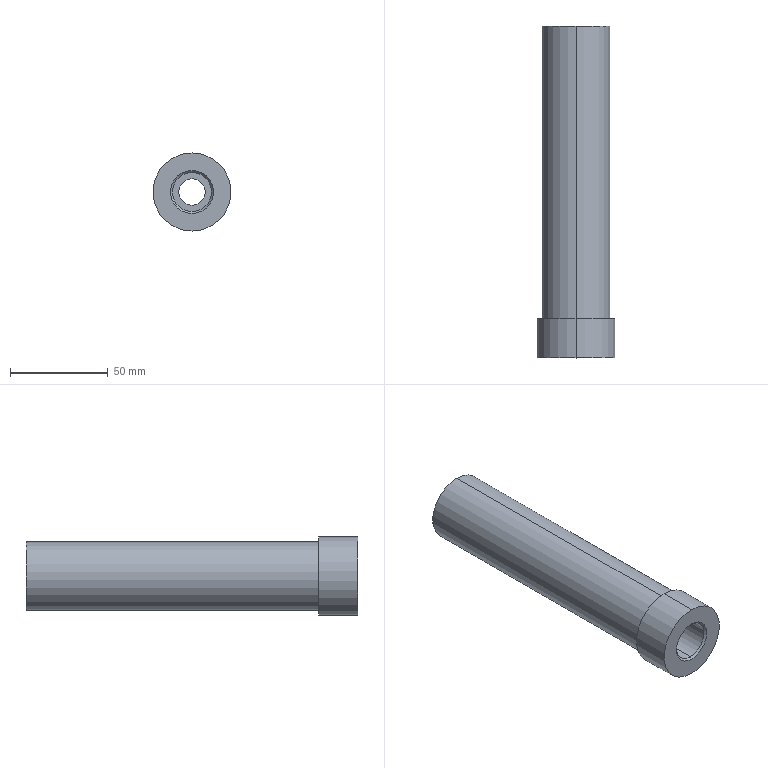Part | STEP file | 1 solid | 14 faces | box 40 x 170 x 40 mm | volume 118148 mm3 | cylinder 8 | plane 4 | cone 2 | commonest cylinder face diameters 13.5 x2 20 x2 35 x2 40 x2
STEP:
#1=CARTESIAN_POINT('',(0.,0.,0.));
#2=DIRECTION('',(0.,0.,1.));
#3=DIRECTION('',(1.,0.,0.));
#4=AXIS2_PLACEMENT_3D('',#1,#2,#3);
#5=CARTESIAN_POINT('',(-72.862,-219.,163.53));
#6=VERTEX_POINT('',#5);
#7=CARTESIAN_POINT('',(-72.862,-220.,162.53));
#8=VERTEX_POINT('',#7);
#9=CARTESIAN_POINT('',(-72.862,-220.,162.53));
#10=DIRECTION('',(0.,-0.7071,-0.7071));
#11=VECTOR('',#10,1.);
#12=LINE('',#9,#11);
#13=CARTESIAN_POINT('',(-72.862,-220.,173.53));
#14=DIRECTION('',(0.,-1.,0.));
#15=DIRECTION('',(0.,0.,-1.));
#16=AXIS2_PLACEMENT_3D('',#13,#14,#15);
#17=CONICAL_SURFACE('',#16,11.,0.7854);
#18=CARTESIAN_POINT('',(6.283,0.));
#19=DIRECTION('',(0.,1.));
#20=VECTOR('',#19,1.);
#21=LINE('',#18,#20);
#22=(GEOMETRIC_REPRESENTATION_CONTEXT(2)PARAMETRIC_REPRESENTATION_CONTEXT()REPRESENTATION_CONTEXT('',''));
#23=DEFINITIONAL_REPRESENTATION('',(#21),#22);
#24=PCURVE('',#17,#23);
#25=CARTESIAN_POINT('',(-72.862,-220.,173.53));
#26=DIRECTION('',(0.,-1.,0.));
#27=DIRECTION('',(0.,0.,-1.));
#28=AXIS2_PLACEMENT_3D('',#25,#26,#27);
#29=CONICAL_SURFACE('',#28,11.,0.7854);
#30=CARTESIAN_POINT('',(0.,0.));
#31=DIRECTION('',(0.,1.));
#32=VECTOR('',#31,1.);
#33=LINE('',#30,#32);
#34=(GEOMETRIC_REPRESENTATION_CONTEXT(2)PARAMETRIC_REPRESENTATION_CONTEXT()REPRESENTATION_CONTEXT('',''));
#35=DEFINITIONAL_REPRESENTATION('',(#33),#34);
#36=PCURVE('',#29,#35);
#37=SURFACE_CURVE('',#12,(#24,#36),.PCURVE_S1.);
#38=EDGE_CURVE('',#6,#8,#37,.T.);
#39=ORIENTED_EDGE('',*,*,#38,.T.);
#40=CARTESIAN_POINT('',(-72.862,-220.,184.53));
#41=VERTEX_POINT('',#40);
#42=CARTESIAN_POINT('',(-72.862,-220.,173.53));
#43=DIRECTION('',(0.,1.,0.));
#44=DIRECTION('',(0.,0.,-1.));
#45=AXIS2_PLACEMENT_3D('',#42,#43,#44);
#46=CIRCLE('',#45,11.);
#47=CARTESIAN_POINT('',(6.283,0.));
#48=DIRECTION('',(-1.,0.));
#49=VECTOR('',#48,1.);
#50=LINE('',#47,#49);
#51=(GEOMETRIC_REPRESENTATION_CONTEXT(2)PARAMETRIC_REPRESENTATION_CONTEXT()REPRESENTATION_CONTEXT('',''));
#52=DEFINITIONAL_REPRESENTATION('',(#50),#51);
#53=PCURVE('',#17,#52);
#54=CARTESIAN_POINT('',(-72.862,-220.,173.53));
#55=DIRECTION('',(0.,-1.,0.));
#56=DIRECTION('',(0.,0.,-1.));
#57=AXIS2_PLACEMENT_3D('',#54,#55,#56);
#58=PLANE('',#57);
#59=CARTESIAN_POINT('',(11.,0.));
#60=CARTESIAN_POINT('',(11.,-19.053));
#61=CARTESIAN_POINT('',(-5.5,-9.526));
#62=CARTESIAN_POINT('',(-22.,0.));
#63=CARTESIAN_POINT('',(-5.5,9.526));
#64=CARTESIAN_POINT('',(11.,19.053));
#65=CARTESIAN_POINT('',(11.,0.));
#66=(BOUNDED_CURVE()B_SPLINE_CURVE(2,(#59,#60,#61,#62,#63,#64,#65),.UNSPECIFIED.,.T.,.F.)B_SPLINE_CURVE_WITH_KNOTS((1,2,2,2,2,1),(-2.094,0.,2.094,4.189,6.283,8.378),.UNSPECIFIED.)CURVE()GEOMETRIC_REPRESENTATION_ITEM()RATIONAL_B_SPLINE_CURVE((1.,0.5,1.,0.5,1.,0.5,1.))REPRESENTATION_ITEM(''));
#67=(GEOMETRIC_REPRESENTATION_CONTEXT(2)PARAMETRIC_REPRESENTATION_CONTEXT()REPRESENTATION_CONTEXT('',''));
#68=DEFINITIONAL_REPRESENTATION('',(#66),#67);
#69=PCURVE('',#58,#68);
#70=SURFACE_CURVE('',#46,(#53,#69),.PCURVE_S1.);
#71=EDGE_CURVE('',#8,#41,#70,.T.);
#72=ORIENTED_EDGE('',*,*,#71,.T.);
#73=CARTESIAN_POINT('',(-72.862,-219.,183.53));
#74=VERTEX_POINT('',#73);
#75=CARTESIAN_POINT('',(-72.862,-220.,184.53));
#76=DIRECTION('',(0.,-0.7071,0.7071));
#77=VECTOR('',#76,1.);
#78=LINE('',#75,#77);
#79=CARTESIAN_POINT('',(3.142,0.));
#80=DIRECTION('',(0.,1.));
#81=VECTOR('',#80,1.);
#82=LINE('',#79,#81);
#83=(GEOMETRIC_REPRESENTATION_CONTEXT(2)PARAMETRIC_REPRESENTATION_CONTEXT()REPRESENTATION_CONTEXT('',''));
#84=DEFINITIONAL_REPRESENTATION('',(#82),#83);
#85=PCURVE('',#17,#84);
#86=CARTESIAN_POINT('',(3.142,0.));
#87=DIRECTION('',(0.,1.));
#88=VECTOR('',#87,1.);
#89=LINE('',#86,#88);
#90=(GEOMETRIC_REPRESENTATION_CONTEXT(2)PARAMETRIC_REPRESENTATION_CONTEXT()REPRESENTATION_CONTEXT('',''));
#91=DEFINITIONAL_REPRESENTATION('',(#89),#90);
#92=PCURVE('',#29,#91);
#93=SURFACE_CURVE('',#78,(#85,#92),.PCURVE_S1.);
#94=EDGE_CURVE('',#74,#41,#93,.T.);
#95=ORIENTED_EDGE('',*,*,#94,.F.);
#96=CARTESIAN_POINT('',(-72.862,-219.,173.53));
#97=DIRECTION('',(0.,-1.,0.));
#98=DIRECTION('',(0.,0.,-1.));
#99=AXIS2_PLACEMENT_3D('',#96,#97,#98);
#100=CIRCLE('',#99,10.);
#101=CARTESIAN_POINT('',(0.,-1.));
#102=DIRECTION('',(1.,0.));
#103=VECTOR('',#102,1.);
#104=LINE('',#101,#103);
#105=(GEOMETRIC_REPRESENTATION_CONTEXT(2)PARAMETRIC_REPRESENTATION_CONTEXT()REPRESENTATION_CONTEXT('',''));
#106=DEFINITIONAL_REPRESENTATION('',(#104),#105);
#107=PCURVE('',#17,#106);
#108=CARTESIAN_POINT('',(-72.862,-220.,173.53));
#109=DIRECTION('',(0.,1.,0.));
#110=DIRECTION('',(0.,0.,1.));
#111=AXIS2_PLACEMENT_3D('',#108,#109,#110);
#112=CYLINDRICAL_SURFACE('',#111,10.);
#113=CARTESIAN_POINT('',(9.425,1.));
#114=DIRECTION('',(-1.,0.));
#115=VECTOR('',#114,1.);
#116=LINE('',#113,#115);
#117=(GEOMETRIC_REPRESENTATION_CONTEXT(2)PARAMETRIC_REPRESENTATION_CONTEXT()REPRESENTATION_CONTEXT('',''));
#118=DEFINITIONAL_REPRESENTATION('',(#116),#117);
#119=PCURVE('',#112,#118);
#120=SURFACE_CURVE('',#100,(#107,#119),.PCURVE_S1.);
#121=EDGE_CURVE('',#74,#6,#120,.T.);
#122=ORIENTED_EDGE('',*,*,#121,.T.);
#123=EDGE_LOOP('',(#39,#72,#95,#122));
#124=FACE_BOUND('',#123,.F.);
#125=ADVANCED_FACE('',(#124),#17,.F.);
#126=CARTESIAN_POINT('',(-72.862,-62.5,183.53));
#127=VERTEX_POINT('',#126);
#128=CARTESIAN_POINT('',(-72.862,-220.,183.53));
#129=DIRECTION('',(0.,1.,0.));
#130=VECTOR('',#129,1.);
#131=LINE('',#128,#130);
#132=CARTESIAN_POINT('',(6.283,0.));
#133=DIRECTION('',(0.,1.));
#134=VECTOR('',#133,1.);
#135=LINE('',#132,#134);
#136=(GEOMETRIC_REPRESENTATION_CONTEXT(2)PARAMETRIC_REPRESENTATION_CONTEXT()REPRESENTATION_CONTEXT('',''));
#137=DEFINITIONAL_REPRESENTATION('',(#135),#136);
#138=PCURVE('',#112,#137);
#139=CARTESIAN_POINT('',(-72.862,-220.,173.53));
#140=DIRECTION('',(0.,1.,0.));
#141=DIRECTION('',(0.,0.,1.));
#142=AXIS2_PLACEMENT_3D('',#139,#140,#141);
#143=CYLINDRICAL_SURFACE('',#142,10.);
#144=CARTESIAN_POINT('',(0.,0.));
#145=DIRECTION('',(0.,1.));
#146=VECTOR('',#145,1.);
#147=LINE('',#144,#146);
#148=(GEOMETRIC_REPRESENTATION_CONTEXT(2)PARAMETRIC_REPRESENTATION_CONTEXT()REPRESENTATION_CONTEXT('',''));
#149=DEFINITIONAL_REPRESENTATION('',(#147),#148);
#150=PCURVE('',#143,#149);
#151=SURFACE_CURVE('',#131,(#138,#150),.PCURVE_S1.);
#152=EDGE_CURVE('',#74,#127,#151,.T.);
#153=ORIENTED_EDGE('',*,*,#152,.T.);
#154=CARTESIAN_POINT('',(-72.862,-62.5,163.53));
#155=VERTEX_POINT('',#154);
#156=CARTESIAN_POINT('',(-72.862,-62.5,173.53));
#157=DIRECTION('',(0.,-1.,0.));
#158=DIRECTION('',(0.,0.,1.));
#159=AXIS2_PLACEMENT_3D('',#156,#157,#158);
#160=CIRCLE('',#159,10.);
#161=CARTESIAN_POINT('',(6.283,157.5));
#162=DIRECTION('',(-1.,0.));
#163=VECTOR('',#162,1.);
#164=LINE('',#161,#163);
#165=(GEOMETRIC_REPRESENTATION_CONTEXT(2)PARAMETRIC_REPRESENTATION_CONTEXT()REPRESENTATION_CONTEXT('',''));
#166=DEFINITIONAL_REPRESENTATION('',(#164),#165);
#167=PCURVE('',#112,#166);
#168=CARTESIAN_POINT('',(-72.862,-62.5,173.53));
#169=DIRECTION('',(0.,1.,0.));
#170=DIRECTION('',(0.,0.,1.));
#171=AXIS2_PLACEMENT_3D('',#168,#169,#170);
#172=PLANE('',#171);
#173=CARTESIAN_POINT('',(10.,0.));
#174=CARTESIAN_POINT('',(10.,-17.321));
#175=CARTESIAN_POINT('',(-5.,-8.66));
#176=CARTESIAN_POINT('',(-20.,0.));
#177=CARTESIAN_POINT('',(-5.,8.66));
#178=CARTESIAN_POINT('',(10.,17.321));
#179=CARTESIAN_POINT('',(10.,0.));
#180=(BOUNDED_CURVE()B_SPLINE_CURVE(2,(#173,#174,#175,#176,#177,#178,#179),.UNSPECIFIED.,.T.,.F.)B_SPLINE_CURVE_WITH_KNOTS((1,2,2,2,2,1),(-2.094,0.,2.094,4.189,6.283,8.378),.UNSPECIFIED.)CURVE()GEOMETRIC_REPRESENTATION_ITEM()RATIONAL_B_SPLINE_CURVE((1.,0.5,1.,0.5,1.,0.5,1.))REPRESENTATION_ITEM(''));
#181=(GEOMETRIC_REPRESENTATION_CONTEXT(2)PARAMETRIC_REPRESENTATION_CONTEXT()REPRESENTATION_CONTEXT('',''));
#182=DEFINITIONAL_REPRESENTATION('',(#180),#181);
#183=PCURVE('',#172,#182);
#184=SURFACE_CURVE('',#160,(#167,#183),.PCURVE_S1.);
#185=EDGE_CURVE('',#127,#155,#184,.T.);
#186=ORIENTED_EDGE('',*,*,#185,.T.);
#187=CARTESIAN_POINT('',(-72.862,-220.,163.53));
#188=DIRECTION('',(0.,1.,0.));
#189=VECTOR('',#188,1.);
#190=LINE('',#187,#189);
#191=CARTESIAN_POINT('',(3.142,0.));
#192=DIRECTION('',(0.,1.));
#193=VECTOR('',#192,1.);
#194=LINE('',#191,#193);
#195=(GEOMETRIC_REPRESENTATION_CONTEXT(2)PARAMETRIC_REPRESENTATION_CONTEXT()REPRESENTATION_CONTEXT('',''));
#196=DEFINITIONAL_REPRESENTATION('',(#194),#195);
#197=PCURVE('',#112,#196);
#198=CARTESIAN_POINT('',(3.142,0.));
#199=DIRECTION('',(0.,1.));
#200=VECTOR('',#199,1.);
#201=LINE('',#198,#200);
#202=(GEOMETRIC_REPRESENTATION_CONTEXT(2)PARAMETRIC_REPRESENTATION_CONTEXT()REPRESENTATION_CONTEXT('',''));
#203=DEFINITIONAL_REPRESENTATION('',(#201),#202);
#204=PCURVE('',#143,#203);
#205=SURFACE_CURVE('',#190,(#197,#204),.PCURVE_S1.);
#206=EDGE_CURVE('',#6,#155,#205,.T.);
#207=ORIENTED_EDGE('',*,*,#206,.F.);
#208=ORIENTED_EDGE('',*,*,#121,.F.);
#209=EDGE_LOOP('',(#153,#186,#207,#208));
#210=FACE_BOUND('',#209,.F.);
#211=ADVANCED_FACE('',(#210),#112,.F.);
#212=CARTESIAN_POINT('',(-72.862,-62.5,180.28));
#213=VERTEX_POINT('',#212);
#214=CARTESIAN_POINT('',(-72.862,-50.,180.28));
#215=VERTEX_POINT('',#214);
#216=CARTESIAN_POINT('',(-72.862,-220.,180.28));
#217=DIRECTION('',(0.,1.,0.));
#218=VECTOR('',#217,1.);
#219=LINE('',#216,#218);
#220=CARTESIAN_POINT('',(-72.862,-220.,173.53));
#221=DIRECTION('',(0.,1.,0.));
#222=DIRECTION('',(0.,0.,1.));
#223=AXIS2_PLACEMENT_3D('',#220,#221,#222);
#224=CYLINDRICAL_SURFACE('',#223,6.75);
#225=CARTESIAN_POINT('',(6.283,0.));
#226=DIRECTION('',(0.,1.));
#227=VECTOR('',#226,1.);
#228=LINE('',#225,#227);
#229=(GEOMETRIC_REPRESENTATION_CONTEXT(2)PARAMETRIC_REPRESENTATION_CONTEXT()REPRESENTATION_CONTEXT('',''));
#230=DEFINITIONAL_REPRESENTATION('',(#228),#229);
#231=PCURVE('',#224,#230);
#232=CARTESIAN_POINT('',(-72.862,-220.,173.53));
#233=DIRECTION('',(0.,1.,0.));
#234=DIRECTION('',(0.,0.,1.));
#235=AXIS2_PLACEMENT_3D('',#232,#233,#234);
#236=CYLINDRICAL_SURFACE('',#235,6.75);
#237=CARTESIAN_POINT('',(0.,0.));
#238=DIRECTION('',(0.,1.));
#239=VECTOR('',#238,1.);
#240=LINE('',#237,#239);
#241=(GEOMETRIC_REPRESENTATION_CONTEXT(2)PARAMETRIC_REPRESENTATION_CONTEXT()REPRESENTATION_CONTEXT('',''));
#242=DEFINITIONAL_REPRESENTATION('',(#240),#241);
#243=PCURVE('',#236,#242);
#244=SURFACE_CURVE('',#219,(#231,#243),.PCURVE_S1.);
#245=EDGE_CURVE('',#213,#215,#244,.T.);
#246=ORIENTED_EDGE('',*,*,#245,.T.);
#247=CARTESIAN_POINT('',(-72.862,-50.,166.78));
#248=VERTEX_POINT('',#247);
#249=CARTESIAN_POINT('',(-72.862,-50.,173.53));
#250=DIRECTION('',(0.,1.,0.));
#251=DIRECTION('',(0.,0.,1.));
#252=AXIS2_PLACEMENT_3D('',#249,#250,#251);
#253=CIRCLE('',#252,6.75);
#254=CARTESIAN_POINT('',(0.,170.));
#255=DIRECTION('',(1.,0.));
#256=VECTOR('',#255,1.);
#257=LINE('',#254,#256);
#258=(GEOMETRIC_REPRESENTATION_CONTEXT(2)PARAMETRIC_REPRESENTATION_CONTEXT()REPRESENTATION_CONTEXT('',''));
#259=DEFINITIONAL_REPRESENTATION('',(#257),#258);
#260=PCURVE('',#224,#259);
#261=CARTESIAN_POINT('',(-72.862,-50.,173.53));
#262=DIRECTION('',(0.,1.,0.));
#263=DIRECTION('',(0.,0.,1.));
#264=AXIS2_PLACEMENT_3D('',#261,#262,#263);
#265=PLANE('',#264);
#266=CARTESIAN_POINT('',(0.,0.));
#267=DIRECTION('',(1.,0.));
#268=AXIS2_PLACEMENT_2D('',#266,#267);
#269=CIRCLE('',#268,6.75);
#270=(GEOMETRIC_REPRESENTATION_CONTEXT(2)PARAMETRIC_REPRESENTATION_CONTEXT()REPRESENTATION_CONTEXT('',''));
#271=DEFINITIONAL_REPRESENTATION('',(#269),#270);
#272=PCURVE('',#265,#271);
#273=SURFACE_CURVE('',#253,(#260,#272),.PCURVE_S1.);
#274=EDGE_CURVE('',#248,#215,#273,.T.);
#275=ORIENTED_EDGE('',*,*,#274,.F.);
#276=CARTESIAN_POINT('',(-72.862,-62.5,166.78));
#277=VERTEX_POINT('',#276);
#278=CARTESIAN_POINT('',(-72.862,-220.,166.78));
#279=DIRECTION('',(0.,1.,0.));
#280=VECTOR('',#279,1.);
#281=LINE('',#278,#280);
#282=CARTESIAN_POINT('',(3.142,0.));
#283=DIRECTION('',(0.,1.));
#284=VECTOR('',#283,1.);
#285=LINE('',#282,#284);
#286=(GEOMETRIC_REPRESENTATION_CONTEXT(2)PARAMETRIC_REPRESENTATION_CONTEXT()REPRESENTATION_CONTEXT('',''));
#287=DEFINITIONAL_REPRESENTATION('',(#285),#286);
#288=PCURVE('',#224,#287);
#289=CARTESIAN_POINT('',(3.142,0.));
#290=DIRECTION('',(0.,1.));
#291=VECTOR('',#290,1.);
#292=LINE('',#289,#291);
#293=(GEOMETRIC_REPRESENTATION_CONTEXT(2)PARAMETRIC_REPRESENTATION_CONTEXT()REPRESENTATION_CONTEXT('',''));
#294=DEFINITIONAL_REPRESENTATION('',(#292),#293);
#295=PCURVE('',#236,#294);
#296=SURFACE_CURVE('',#281,(#288,#295),.PCURVE_S1.);
#297=EDGE_CURVE('',#277,#248,#296,.T.);
#298=ORIENTED_EDGE('',*,*,#297,.F.);
#299=CARTESIAN_POINT('',(-72.862,-62.5,173.53));
#300=DIRECTION('',(0.,-1.,0.));
#301=DIRECTION('',(0.,0.,1.));
#302=AXIS2_PLACEMENT_3D('',#299,#300,#301);
#303=CIRCLE('',#302,6.75);
#304=CARTESIAN_POINT('',(6.283,157.5));
#305=DIRECTION('',(-1.,0.));
#306=VECTOR('',#305,1.);
#307=LINE('',#304,#306);
#308=(GEOMETRIC_REPRESENTATION_CONTEXT(2)PARAMETRIC_REPRESENTATION_CONTEXT()REPRESENTATION_CONTEXT('',''));
#309=DEFINITIONAL_REPRESENTATION('',(#307),#308);
#310=PCURVE('',#224,#309);
#311=CARTESIAN_POINT('',(6.75,0.));
#312=CARTESIAN_POINT('',(6.75,-11.691));
#313=CARTESIAN_POINT('',(-3.375,-5.846));
#314=CARTESIAN_POINT('',(-13.5,0.));
#315=CARTESIAN_POINT('',(-3.375,5.846));
#316=CARTESIAN_POINT('',(6.75,11.691));
#317=CARTESIAN_POINT('',(6.75,0.));
#318=(BOUNDED_CURVE()B_SPLINE_CURVE(2,(#311,#312,#313,#314,#315,#316,#317),.UNSPECIFIED.,.T.,.F.)B_SPLINE_CURVE_WITH_KNOTS((1,2,2,2,2,1),(-2.094,0.,2.094,4.189,6.283,8.378),.UNSPECIFIED.)CURVE()GEOMETRIC_REPRESENTATION_ITEM()RATIONAL_B_SPLINE_CURVE((1.,0.5,1.,0.5,1.,0.5,1.))REPRESENTATION_ITEM(''));
#319=(GEOMETRIC_REPRESENTATION_CONTEXT(2)PARAMETRIC_REPRESENTATION_CONTEXT()REPRESENTATION_CONTEXT('',''));
#320=DEFINITIONAL_REPRESENTATION('',(#318),#319);
#321=PCURVE('',#172,#320);
#322=SURFACE_CURVE('',#303,(#310,#321),.PCURVE_S1.);
#323=EDGE_CURVE('',#213,#277,#322,.T.);
#324=ORIENTED_EDGE('',*,*,#323,.F.);
#325=EDGE_LOOP('',(#246,#275,#298,#324));
#326=FACE_BOUND('',#325,.F.);
#327=ADVANCED_FACE('',(#326),#224,.F.);
#328=CARTESIAN_POINT('',(-72.862,-200.,193.53));
#329=VERTEX_POINT('',#328);
#330=CARTESIAN_POINT('',(-72.862,-200.,153.53));
#331=VERTEX_POINT('',#330);
#332=CARTESIAN_POINT('',(-72.862,-200.,173.53));
#333=DIRECTION('',(0.,1.,0.));
#334=DIRECTION('',(0.,0.,-1.));
#335=AXIS2_PLACEMENT_3D('',#332,#333,#334);
#336=CIRCLE('',#335,20.);
#337=CARTESIAN_POINT('',(-72.862,-50.,173.53));
#338=DIRECTION('',(0.,-1.,0.));
#339=DIRECTION('',(0.,0.,-1.));
#340=AXIS2_PLACEMENT_3D('',#337,#338,#339);
#341=CYLINDRICAL_SURFACE('',#340,20.);
#342=CARTESIAN_POINT('',(6.283,150.));
#343=DIRECTION('',(-1.,0.));
#344=VECTOR('',#343,1.);
#345=LINE('',#342,#344);
#346=(GEOMETRIC_REPRESENTATION_CONTEXT(2)PARAMETRIC_REPRESENTATION_CONTEXT()REPRESENTATION_CONTEXT('',''));
#347=DEFINITIONAL_REPRESENTATION('',(#345),#346);
#348=PCURVE('',#341,#347);
#349=CARTESIAN_POINT('',(-72.862,-200.,48.53));
#350=DIRECTION('',(0.,-1.,0.));
#351=DIRECTION('',(0.,0.,-1.));
#352=AXIS2_PLACEMENT_3D('',#349,#350,#351);
#353=PLANE('',#352);
#354=CARTESIAN_POINT('',(-105.,0.));
#355=CARTESIAN_POINT('',(-105.,-34.641));
#356=CARTESIAN_POINT('',(-135.,-17.321));
#357=CARTESIAN_POINT('',(-165.,0.));
#358=CARTESIAN_POINT('',(-135.,17.321));
#359=CARTESIAN_POINT('',(-105.,34.641));
#360=CARTESIAN_POINT('',(-105.,0.));
#361=(BOUNDED_CURVE()B_SPLINE_CURVE(2,(#354,#355,#356,#357,#358,#359,#360),.UNSPECIFIED.,.T.,.F.)B_SPLINE_CURVE_WITH_KNOTS((1,2,2,2,2,1),(-2.094,0.,2.094,4.189,6.283,8.378),.UNSPECIFIED.)CURVE()GEOMETRIC_REPRESENTATION_ITEM()RATIONAL_B_SPLINE_CURVE((1.,0.5,1.,0.5,1.,0.5,1.))REPRESENTATION_ITEM(''));
#362=(GEOMETRIC_REPRESENTATION_CONTEXT(2)PARAMETRIC_REPRESENTATION_CONTEXT()REPRESENTATION_CONTEXT('',''));
#363=DEFINITIONAL_REPRESENTATION('',(#361),#362);
#364=PCURVE('',#353,#363);
#365=SURFACE_CURVE('',#336,(#348,#364),.PCURVE_S1.);
#366=EDGE_CURVE('',#329,#331,#365,.T.);
#367=ORIENTED_EDGE('',*,*,#366,.F.);
#368=CARTESIAN_POINT('',(-72.862,-220.,193.53));
#369=VERTEX_POINT('',#368);
#370=CARTESIAN_POINT('',(-72.862,-50.,193.53));
#371=DIRECTION('',(0.,-1.,0.));
#372=VECTOR('',#371,1.);
#373=LINE('',#370,#372);
#374=CARTESIAN_POINT('',(3.142,0.));
#375=DIRECTION('',(0.,1.));
#376=VECTOR('',#375,1.);
#377=LINE('',#374,#376);
#378=(GEOMETRIC_REPRESENTATION_CONTEXT(2)PARAMETRIC_REPRESENTATION_CONTEXT()REPRESENTATION_CONTEXT('',''));
#379=DEFINITIONAL_REPRESENTATION('',(#377),#378);
#380=PCURVE('',#341,#379);
#381=CARTESIAN_POINT('',(-72.862,-50.,173.53));
#382=DIRECTION('',(0.,-1.,0.));
#383=DIRECTION('',(0.,0.,-1.));
#384=AXIS2_PLACEMENT_3D('',#381,#382,#383);
#385=CYLINDRICAL_SURFACE('',#384,20.);
#386=CARTESIAN_POINT('',(3.142,0.));
#387=DIRECTION('',(0.,1.));
#388=VECTOR('',#387,1.);
#389=LINE('',#386,#388);
#390=(GEOMETRIC_REPRESENTATION_CONTEXT(2)PARAMETRIC_REPRESENTATION_CONTEXT()REPRESENTATION_CONTEXT('',''));
#391=DEFINITIONAL_REPRESENTATION('',(#389),#390);
#392=PCURVE('',#385,#391);
#393=SURFACE_CURVE('',#373,(#380,#392),.PCURVE_S1.);
#394=EDGE_CURVE('',#329,#369,#393,.T.);
#395=ORIENTED_EDGE('',*,*,#394,.T.);
#396=CARTESIAN_POINT('',(-72.862,-220.,153.53));
#397=VERTEX_POINT('',#396);
#398=CARTESIAN_POINT('',(-72.862,-220.,173.53));
#399=DIRECTION('',(0.,-1.,0.));
#400=DIRECTION('',(0.,0.,-1.));
#401=AXIS2_PLACEMENT_3D('',#398,#399,#400);
#402=CIRCLE('',#401,20.);
#403=CARTESIAN_POINT('',(0.,170.));
#404=DIRECTION('',(1.,0.));
#405=VECTOR('',#404,1.);
#406=LINE('',#403,#405);
#407=(GEOMETRIC_REPRESENTATION_CONTEXT(2)PARAMETRIC_REPRESENTATION_CONTEXT()REPRESENTATION_CONTEXT('',''));
#408=DEFINITIONAL_REPRESENTATION('',(#406),#407);
#409=PCURVE('',#341,#408);
#410=CARTESIAN_POINT('',(0.,0.));
#411=DIRECTION('',(1.,0.));
#412=AXIS2_PLACEMENT_2D('',#410,#411);
#413=CIRCLE('',#412,20.);
#414=(GEOMETRIC_REPRESENTATION_CONTEXT(2)PARAMETRIC_REPRESENTATION_CONTEXT()REPRESENTATION_CONTEXT('',''));
#415=DEFINITIONAL_REPRESENTATION('',(#413),#414);
#416=PCURVE('',#58,#415);
#417=SURFACE_CURVE('',#402,(#409,#416),.PCURVE_S1.);
#418=EDGE_CURVE('',#397,#369,#417,.T.);
#419=ORIENTED_EDGE('',*,*,#418,.F.);
#420=CARTESIAN_POINT('',(-72.862,-50.,153.53));
#421=DIRECTION('',(0.,-1.,0.));
#422=VECTOR('',#421,1.);
#423=LINE('',#420,#422);
#424=CARTESIAN_POINT('',(0.,0.));
#425=DIRECTION('',(0.,1.));
#426=VECTOR('',#425,1.);
#427=LINE('',#424,#426);
#428=(GEOMETRIC_REPRESENTATION_CONTEXT(2)PARAMETRIC_REPRESENTATION_CONTEXT()REPRESENTATION_CONTEXT('',''));
#429=DEFINITIONAL_REPRESENTATION('',(#427),#428);
#430=PCURVE('',#341,#429);
#431=CARTESIAN_POINT('',(6.283,0.));
#432=DIRECTION('',(0.,1.));
#433=VECTOR('',#432,1.);
#434=LINE('',#431,#433);
#435=(GEOMETRIC_REPRESENTATION_CONTEXT(2)PARAMETRIC_REPRESENTATION_CONTEXT()REPRESENTATION_CONTEXT('',''));
#436=DEFINITIONAL_REPRESENTATION('',(#434),#435);
#437=PCURVE('',#385,#436);
#438=SURFACE_CURVE('',#423,(#430,#437),.PCURVE_S1.);
#439=EDGE_CURVE('',#331,#397,#438,.T.);
#440=ORIENTED_EDGE('',*,*,#439,.F.);
#441=EDGE_LOOP('',(#367,#395,#419,#440));
#442=FACE_BOUND('',#441,.T.);
#443=ADVANCED_FACE('',(#442),#341,.T.);
#444=CARTESIAN_POINT('',(-72.862,-50.,156.03));
#445=VERTEX_POINT('',#444);
#446=CARTESIAN_POINT('',(-72.862,-50.,191.03));
#447=VERTEX_POINT('',#446);
#448=CARTESIAN_POINT('',(-72.862,-50.,173.53));
#449=DIRECTION('',(0.,-1.,0.));
#450=DIRECTION('',(0.,0.,1.));
#451=AXIS2_PLACEMENT_3D('',#448,#449,#450);
#452=CIRCLE('',#451,17.5);
#453=CARTESIAN_POINT('',(-72.862,-50.,173.53));
#454=DIRECTION('',(0.,-1.,0.));
#455=DIRECTION('',(0.,0.,-1.));
#456=AXIS2_PLACEMENT_3D('',#453,#454,#455);
#457=CYLINDRICAL_SURFACE('',#456,17.5);
#458=CARTESIAN_POINT('',(-3.142,0.));
#459=DIRECTION('',(1.,0.));
#460=VECTOR('',#459,1.);
#461=LINE('',#458,#460);
#462=(GEOMETRIC_REPRESENTATION_CONTEXT(2)PARAMETRIC_REPRESENTATION_CONTEXT()REPRESENTATION_CONTEXT('',''));
#463=DEFINITIONAL_REPRESENTATION('',(#461),#462);
#464=PCURVE('',#457,#463);
#465=CARTESIAN_POINT('',(17.5,0.));
#466=CARTESIAN_POINT('',(17.5,-30.311));
#467=CARTESIAN_POINT('',(-8.75,-15.155));
#468=CARTESIAN_POINT('',(-35.,0.));
#469=CARTESIAN_POINT('',(-8.75,15.155));
#470=CARTESIAN_POINT('',(17.5,30.311));
#471=CARTESIAN_POINT('',(17.5,0.));
#472=(BOUNDED_CURVE()B_SPLINE_CURVE(2,(#465,#466,#467,#468,#469,#470,#471),.UNSPECIFIED.,.T.,.F.)B_SPLINE_CURVE_WITH_KNOTS((1,2,2,2,2,1),(-2.094,0.,2.094,4.189,6.283,8.378),.UNSPECIFIED.)CURVE()GEOMETRIC_REPRESENTATION_ITEM()RATIONAL_B_SPLINE_CURVE((1.,0.5,1.,0.5,1.,0.5,1.))REPRESENTATION_ITEM(''));
#473=(GEOMETRIC_REPRESENTATION_CONTEXT(2)PARAMETRIC_REPRESENTATION_CONTEXT()REPRESENTATION_CONTEXT('',''));
#474=DEFINITIONAL_REPRESENTATION('',(#472),#473);
#475=PCURVE('',#265,#474);
#476=SURFACE_CURVE('',#452,(#464,#475),.PCURVE_S1.);
#477=EDGE_CURVE('',#445,#447,#476,.T.);
#478=ORIENTED_EDGE('',*,*,#477,.T.);
#479=CARTESIAN_POINT('',(-72.862,-200.,191.03));
#480=VERTEX_POINT('',#479);
#481=CARTESIAN_POINT('',(-72.862,-50.,191.03));
#482=DIRECTION('',(0.,-1.,0.));
#483=VECTOR('',#482,1.);
#484=LINE('',#481,#483);
#485=CARTESIAN_POINT('',(3.142,0.));
#486=DIRECTION('',(0.,1.));
#487=VECTOR('',#486,1.);
#488=LINE('',#485,#487);
#489=(GEOMETRIC_REPRESENTATION_CONTEXT(2)PARAMETRIC_REPRESENTATION_CONTEXT()REPRESENTATION_CONTEXT('',''));
#490=DEFINITIONAL_REPRESENTATION('',(#488),#489);
#491=PCURVE('',#457,#490);
#492=CARTESIAN_POINT('',(-72.862,-50.,173.53));
#493=DIRECTION('',(0.,-1.,0.));
#494=DIRECTION('',(0.,0.,-1.));
#495=AXIS2_PLACEMENT_3D('',#492,#493,#494);
#496=CYLINDRICAL_SURFACE('',#495,17.5);
#497=CARTESIAN_POINT('',(3.142,0.));
#498=DIRECTION('',(0.,1.));
#499=VECTOR('',#498,1.);
#500=LINE('',#497,#499);
#501=(GEOMETRIC_REPRESENTATION_CONTEXT(2)PARAMETRIC_REPRESENTATION_CONTEXT()REPRESENTATION_CONTEXT('',''));
#502=DEFINITIONAL_REPRESENTATION('',(#500),#501);
#503=PCURVE('',#496,#502);
#504=SURFACE_CURVE('',#484,(#491,#503),.PCURVE_S1.);
#505=EDGE_CURVE('',#447,#480,#504,.T.);
#506=ORIENTED_EDGE('',*,*,#505,.T.);
#507=CARTESIAN_POINT('',(-72.862,-200.,156.03));
#508=VERTEX_POINT('',#507);
#509=CARTESIAN_POINT('',(-72.862,-200.,173.53));
#510=DIRECTION('',(0.,1.,0.));
#511=DIRECTION('',(0.,0.,-1.));
#512=AXIS2_PLACEMENT_3D('',#509,#510,#511);
#513=CIRCLE('',#512,17.5);
#514=CARTESIAN_POINT('',(6.283,150.));
#515=DIRECTION('',(-1.,0.));
#516=VECTOR('',#515,1.);
#517=LINE('',#514,#516);
#518=(GEOMETRIC_REPRESENTATION_CONTEXT(2)PARAMETRIC_REPRESENTATION_CONTEXT()REPRESENTATION_CONTEXT('',''));
#519=DEFINITIONAL_REPRESENTATION('',(#517),#518);
#520=PCURVE('',#457,#519);
#521=CARTESIAN_POINT('',(-107.5,0.));
#522=CARTESIAN_POINT('',(-107.5,-30.311));
#523=CARTESIAN_POINT('',(-133.75,-15.155));
#524=CARTESIAN_POINT('',(-160.,0.));
#525=CARTESIAN_POINT('',(-133.75,15.155));
#526=CARTESIAN_POINT('',(-107.5,30.311));
#527=CARTESIAN_POINT('',(-107.5,0.));
#528=(BOUNDED_CURVE()B_SPLINE_CURVE(2,(#521,#522,#523,#524,#525,#526,#527),.UNSPECIFIED.,.T.,.F.)B_SPLINE_CURVE_WITH_KNOTS((1,2,2,2,2,1),(-2.094,0.,2.094,4.189,6.283,8.378),.UNSPECIFIED.)CURVE()GEOMETRIC_REPRESENTATION_ITEM()RATIONAL_B_SPLINE_CURVE((1.,0.5,1.,0.5,1.,0.5,1.))REPRESENTATION_ITEM(''));
#529=(GEOMETRIC_REPRESENTATION_CONTEXT(2)PARAMETRIC_REPRESENTATION_CONTEXT()REPRESENTATION_CONTEXT('',''));
#530=DEFINITIONAL_REPRESENTATION('',(#528),#529);
#531=PCURVE('',#353,#530);
#532=SURFACE_CURVE('',#513,(#520,#531),.PCURVE_S1.);
#533=EDGE_CURVE('',#480,#508,#532,.T.);
#534=ORIENTED_EDGE('',*,*,#533,.T.);
#535=CARTESIAN_POINT('',(-72.862,-50.,156.03));
#536=DIRECTION('',(0.,-1.,0.));
#537=VECTOR('',#536,1.);
#538=LINE('',#535,#537);
#539=CARTESIAN_POINT('',(0.,0.));
#540=DIRECTION('',(0.,1.));
#541=VECTOR('',#540,1.);
#542=LINE('',#539,#541);
#543=(GEOMETRIC_REPRESENTATION_CONTEXT(2)PARAMETRIC_REPRESENTATION_CONTEXT()REPRESENTATION_CONTEXT('',''));
#544=DEFINITIONAL_REPRESENTATION('',(#542),#543);
#545=PCURVE('',#457,#544);
#546=CARTESIAN_POINT('',(6.283,0.));
#547=DIRECTION('',(0.,1.));
#548=VECTOR('',#547,1.);
#549=LINE('',#546,#548);
#550=(GEOMETRIC_REPRESENTATION_CONTEXT(2)PARAMETRIC_REPRESENTATION_CONTEXT()REPRESENTATION_CONTEXT('',''));
#551=DEFINITIONAL_REPRESENTATION('',(#549),#550);
#552=PCURVE('',#496,#551);
#553=SURFACE_CURVE('',#538,(#545,#552),.PCURVE_S1.);
#554=EDGE_CURVE('',#445,#508,#553,.T.);
#555=ORIENTED_EDGE('',*,*,#554,.F.);
#556=EDGE_LOOP('',(#478,#506,#534,#555));
#557=FACE_BOUND('',#556,.T.);
#558=ADVANCED_FACE('',(#557),#457,.T.);
#559=CARTESIAN_POINT('',(-72.862,-50.,173.53));
#560=DIRECTION('',(0.,1.,0.));
#561=DIRECTION('',(0.,0.,1.));
#562=AXIS2_PLACEMENT_3D('',#559,#560,#561);
#563=CIRCLE('',#562,6.75);
#564=CARTESIAN_POINT('',(0.,0.));
#565=DIRECTION('',(1.,0.));
#566=AXIS2_PLACEMENT_2D('',#564,#565);
#567=CIRCLE('',#566,6.75);
#568=(GEOMETRIC_REPRESENTATION_CONTEXT(2)PARAMETRIC_REPRESENTATION_CONTEXT()REPRESENTATION_CONTEXT('',''));
#569=DEFINITIONAL_REPRESENTATION('',(#567),#568);
#570=PCURVE('',#265,#569);
#571=CARTESIAN_POINT('',(0.,170.));
#572=DIRECTION('',(1.,0.));
#573=VECTOR('',#572,1.);
#574=LINE('',#571,#573);
#575=(GEOMETRIC_REPRESENTATION_CONTEXT(2)PARAMETRIC_REPRESENTATION_CONTEXT()REPRESENTATION_CONTEXT('',''));
#576=DEFINITIONAL_REPRESENTATION('',(#574),#575);
#577=PCURVE('',#236,#576);
#578=SURFACE_CURVE('',#563,(#570,#577),.PCURVE_S1.);
#579=EDGE_CURVE('',#215,#248,#578,.T.);
#580=ORIENTED_EDGE('',*,*,#579,.F.);
#581=ORIENTED_EDGE('',*,*,#274,.F.);
#582=EDGE_LOOP('',(#580,#581));
#583=FACE_BOUND('',#582,.T.);
#584=ORIENTED_EDGE('',*,*,#477,.F.);
#585=CARTESIAN_POINT('',(-72.862,-50.,173.53));
#586=DIRECTION('',(0.,-1.,0.));
#587=DIRECTION('',(0.,0.,1.));
#588=AXIS2_PLACEMENT_3D('',#585,#586,#587);
#589=CIRCLE('',#588,17.5);
#590=CARTESIAN_POINT('',(17.5,0.));
#591=CARTESIAN_POINT('',(17.5,-30.311));
#592=CARTESIAN_POINT('',(-8.75,-15.155));
#593=CARTESIAN_POINT('',(-35.,0.));
#594=CARTESIAN_POINT('',(-8.75,15.155));
#595=CARTESIAN_POINT('',(17.5,30.311));
#596=CARTESIAN_POINT('',(17.5,0.));
#597=(BOUNDED_CURVE()B_SPLINE_CURVE(2,(#590,#591,#592,#593,#594,#595,#596),.UNSPECIFIED.,.T.,.F.)B_SPLINE_CURVE_WITH_KNOTS((1,2,2,2,2,1),(-2.094,0.,2.094,4.189,6.283,8.378),.UNSPECIFIED.)CURVE()GEOMETRIC_REPRESENTATION_ITEM()RATIONAL_B_SPLINE_CURVE((1.,0.5,1.,0.5,1.,0.5,1.))REPRESENTATION_ITEM(''));
#598=(GEOMETRIC_REPRESENTATION_CONTEXT(2)PARAMETRIC_REPRESENTATION_CONTEXT()REPRESENTATION_CONTEXT('',''));
#599=DEFINITIONAL_REPRESENTATION('',(#597),#598);
#600=PCURVE('',#265,#599);
#601=CARTESIAN_POINT('',(3.142,0.));
#602=DIRECTION('',(1.,0.));
#603=VECTOR('',#602,1.);
#604=LINE('',#601,#603);
#605=(GEOMETRIC_REPRESENTATION_CONTEXT(2)PARAMETRIC_REPRESENTATION_CONTEXT()REPRESENTATION_CONTEXT('',''));
#606=DEFINITIONAL_REPRESENTATION('',(#604),#605);
#607=PCURVE('',#496,#606);
#608=SURFACE_CURVE('',#589,(#600,#607),.PCURVE_S1.);
#609=EDGE_CURVE('',#447,#445,#608,.T.);
#610=ORIENTED_EDGE('',*,*,#609,.F.);
#611=EDGE_LOOP('',(#584,#610));
#612=FACE_BOUND('',#611,.T.);
#613=ADVANCED_FACE('',(#583,#612),#265,.T.);
#614=ORIENTED_EDGE('',*,*,#505,.F.);
#615=ORIENTED_EDGE('',*,*,#609,.T.);
#616=ORIENTED_EDGE('',*,*,#554,.T.);
#617=CARTESIAN_POINT('',(-72.862,-200.,173.53));
#618=DIRECTION('',(0.,1.,0.));
#619=DIRECTION('',(0.,0.,-1.));
#620=AXIS2_PLACEMENT_3D('',#617,#618,#619);
#621=CIRCLE('',#620,17.5);
#622=CARTESIAN_POINT('',(6.283,150.));
#623=DIRECTION('',(-1.,0.));
#624=VECTOR('',#623,1.);
#625=LINE('',#622,#624);
#626=(GEOMETRIC_REPRESENTATION_CONTEXT(2)PARAMETRIC_REPRESENTATION_CONTEXT()REPRESENTATION_CONTEXT('',''));
#627=DEFINITIONAL_REPRESENTATION('',(#625),#626);
#628=PCURVE('',#496,#627);
#629=CARTESIAN_POINT('',(-107.5,0.));
#630=CARTESIAN_POINT('',(-107.5,-30.311));
#631=CARTESIAN_POINT('',(-133.75,-15.155));
#632=CARTESIAN_POINT('',(-160.,0.));
#633=CARTESIAN_POINT('',(-133.75,15.155));
#634=CARTESIAN_POINT('',(-107.5,30.311));
#635=CARTESIAN_POINT('',(-107.5,0.));
#636=(BOUNDED_CURVE()B_SPLINE_CURVE(2,(#629,#630,#631,#632,#633,#634,#635),.UNSPECIFIED.,.T.,.F.)B_SPLINE_CURVE_WITH_KNOTS((1,2,2,2,2,1),(-2.094,0.,2.094,4.189,6.283,8.378),.UNSPECIFIED.)CURVE()GEOMETRIC_REPRESENTATION_ITEM()RATIONAL_B_SPLINE_CURVE((1.,0.5,1.,0.5,1.,0.5,1.))REPRESENTATION_ITEM(''));
#637=(GEOMETRIC_REPRESENTATION_CONTEXT(2)PARAMETRIC_REPRESENTATION_CONTEXT()REPRESENTATION_CONTEXT('',''));
#638=DEFINITIONAL_REPRESENTATION('',(#636),#637);
#639=PCURVE('',#353,#638);
#640=SURFACE_CURVE('',#621,(#628,#639),.PCURVE_S1.);
#641=EDGE_CURVE('',#508,#480,#640,.T.);
#642=ORIENTED_EDGE('',*,*,#641,.T.);
#643=EDGE_LOOP('',(#614,#615,#616,#642));
#644=FACE_BOUND('',#643,.T.);
#645=ADVANCED_FACE('',(#644),#496,.T.);
#646=ORIENTED_EDGE('',*,*,#71,.T.);
#647=CARTESIAN_POINT('',(-72.862,-220.,173.53));
#648=DIRECTION('',(0.,1.,0.));
#649=DIRECTION('',(0.,0.,-1.));
#650=AXIS2_PLACEMENT_3D('',#647,#648,#649);
#651=CIRCLE('',#650,11.);
#652=CARTESIAN_POINT('',(11.,0.));
#653=CARTESIAN_POINT('',(11.,-19.053));
#654=CARTESIAN_POINT('',(-5.5,-9.526));
#655=CARTESIAN_POINT('',(-22.,0.));
#656=CARTESIAN_POINT('',(-5.5,9.526));
#657=CARTESIAN_POINT('',(11.,19.053));
#658=CARTESIAN_POINT('',(11.,0.));
#659=(BOUNDED_CURVE()B_SPLINE_CURVE(2,(#652,#653,#654,#655,#656,#657,#658),.UNSPECIFIED.,.T.,.F.)B_SPLINE_CURVE_WITH_KNOTS((1,2,2,2,2,1),(-2.094,0.,2.094,4.189,6.283,8.378),.UNSPECIFIED.)CURVE()GEOMETRIC_REPRESENTATION_ITEM()RATIONAL_B_SPLINE_CURVE((1.,0.5,1.,0.5,1.,0.5,1.))REPRESENTATION_ITEM(''));
#660=(GEOMETRIC_REPRESENTATION_CONTEXT(2)PARAMETRIC_REPRESENTATION_CONTEXT()REPRESENTATION_CONTEXT('',''));
#661=DEFINITIONAL_REPRESENTATION('',(#659),#660);
#662=PCURVE('',#58,#661);
#663=CARTESIAN_POINT('',(6.283,0.));
#664=DIRECTION('',(-1.,0.));
#665=VECTOR('',#664,1.);
#666=LINE('',#663,#665);
#667=(GEOMETRIC_REPRESENTATION_CONTEXT(2)PARAMETRIC_REPRESENTATION_CONTEXT()REPRESENTATION_CONTEXT('',''));
#668=DEFINITIONAL_REPRESENTATION('',(#666),#667);
#669=PCURVE('',#29,#668);
#670=SURFACE_CURVE('',#651,(#662,#669),.PCURVE_S1.);
#671=EDGE_CURVE('',#41,#8,#670,.T.);
#672=ORIENTED_EDGE('',*,*,#671,.T.);
#673=EDGE_LOOP('',(#646,#672));
#674=FACE_BOUND('',#673,.T.);
#675=ORIENTED_EDGE('',*,*,#418,.T.);
#676=CARTESIAN_POINT('',(-72.862,-220.,173.53));
#677=DIRECTION('',(0.,-1.,0.));
#678=DIRECTION('',(0.,0.,-1.));
#679=AXIS2_PLACEMENT_3D('',#676,#677,#678);
#680=CIRCLE('',#679,20.);
#681=CARTESIAN_POINT('',(0.,0.));
#682=DIRECTION('',(1.,0.));
#683=AXIS2_PLACEMENT_2D('',#681,#682);
#684=CIRCLE('',#683,20.);
#685=(GEOMETRIC_REPRESENTATION_CONTEXT(2)PARAMETRIC_REPRESENTATION_CONTEXT()REPRESENTATION_CONTEXT('',''));
#686=DEFINITIONAL_REPRESENTATION('',(#684),#685);
#687=PCURVE('',#58,#686);
#688=CARTESIAN_POINT('',(0.,170.));
#689=DIRECTION('',(1.,0.));
#690=VECTOR('',#689,1.);
#691=LINE('',#688,#690);
#692=(GEOMETRIC_REPRESENTATION_CONTEXT(2)PARAMETRIC_REPRESENTATION_CONTEXT()REPRESENTATION_CONTEXT('',''));
#693=DEFINITIONAL_REPRESENTATION('',(#691),#692);
#694=PCURVE('',#385,#693);
#695=SURFACE_CURVE('',#680,(#687,#694),.PCURVE_S1.);
#696=EDGE_CURVE('',#369,#397,#695,.T.);
#697=ORIENTED_EDGE('',*,*,#696,.T.);
#698=EDGE_LOOP('',(#675,#697));
#699=FACE_BOUND('',#698,.T.);
#700=ADVANCED_FACE('',(#674,#699),#58,.T.);
#701=ORIENTED_EDGE('',*,*,#394,.F.);
#702=CARTESIAN_POINT('',(-72.862,-200.,173.53));
#703=DIRECTION('',(0.,1.,0.));
#704=DIRECTION('',(0.,0.,-1.));
#705=AXIS2_PLACEMENT_3D('',#702,#703,#704);
#706=CIRCLE('',#705,20.);
#707=CARTESIAN_POINT('',(6.283,150.));
#708=DIRECTION('',(-1.,0.));
#709=VECTOR('',#708,1.);
#710=LINE('',#707,#709);
#711=(GEOMETRIC_REPRESENTATION_CONTEXT(2)PARAMETRIC_REPRESENTATION_CONTEXT()REPRESENTATION_CONTEXT('',''));
#712=DEFINITIONAL_REPRESENTATION('',(#710),#711);
#713=PCURVE('',#385,#712);
#714=CARTESIAN_POINT('',(-105.,0.));
#715=CARTESIAN_POINT('',(-105.,-34.641));
#716=CARTESIAN_POINT('',(-135.,-17.321));
#717=CARTESIAN_POINT('',(-165.,0.));
#718=CARTESIAN_POINT('',(-135.,17.321));
#719=CARTESIAN_POINT('',(-105.,34.641));
#720=CARTESIAN_POINT('',(-105.,0.));
#721=(BOUNDED_CURVE()B_SPLINE_CURVE(2,(#714,#715,#716,#717,#718,#719,#720),.UNSPECIFIED.,.T.,.F.)B_SPLINE_CURVE_WITH_KNOTS((1,2,2,2,2,1),(-2.094,0.,2.094,4.189,6.283,8.378),.UNSPECIFIED.)CURVE()GEOMETRIC_REPRESENTATION_ITEM()RATIONAL_B_SPLINE_CURVE((1.,0.5,1.,0.5,1.,0.5,1.))REPRESENTATION_ITEM(''));
#722=(GEOMETRIC_REPRESENTATION_CONTEXT(2)PARAMETRIC_REPRESENTATION_CONTEXT()REPRESENTATION_CONTEXT('',''));
#723=DEFINITIONAL_REPRESENTATION('',(#721),#722);
#724=PCURVE('',#353,#723);
#725=SURFACE_CURVE('',#706,(#713,#724),.PCURVE_S1.);
#726=EDGE_CURVE('',#331,#329,#725,.T.);
#727=ORIENTED_EDGE('',*,*,#726,.F.);
#728=ORIENTED_EDGE('',*,*,#439,.T.);
#729=ORIENTED_EDGE('',*,*,#696,.F.);
#730=EDGE_LOOP('',(#701,#727,#728,#729));
#731=FACE_BOUND('',#730,.T.);
#732=ADVANCED_FACE('',(#731),#385,.T.);
#733=ORIENTED_EDGE('',*,*,#641,.F.);
#734=ORIENTED_EDGE('',*,*,#533,.F.);
#735=EDGE_LOOP('',(#733,#734));
#736=FACE_BOUND('',#735,.T.);
#737=ORIENTED_EDGE('',*,*,#726,.T.);
#738=ORIENTED_EDGE('',*,*,#366,.T.);
#739=EDGE_LOOP('',(#737,#738));
#740=FACE_BOUND('',#739,.T.);
#741=ADVANCED_FACE('',(#736,#740),#353,.F.);
#742=ORIENTED_EDGE('',*,*,#579,.F.);
#743=ORIENTED_EDGE('',*,*,#245,.F.);
#744=CARTESIAN_POINT('',(-72.862,-62.5,173.53));
#745=DIRECTION('',(0.,-1.,0.));
#746=DIRECTION('',(0.,0.,1.));
#747=AXIS2_PLACEMENT_3D('',#744,#745,#746);
#748=CIRCLE('',#747,6.75);
#749=CARTESIAN_POINT('',(6.283,157.5));
#750=DIRECTION('',(-1.,0.));
#751=VECTOR('',#750,1.);
#752=LINE('',#749,#751);
#753=(GEOMETRIC_REPRESENTATION_CONTEXT(2)PARAMETRIC_REPRESENTATION_CONTEXT()REPRESENTATION_CONTEXT('',''));
#754=DEFINITIONAL_REPRESENTATION('',(#752),#753);
#755=PCURVE('',#236,#754);
#756=CARTESIAN_POINT('',(6.75,0.));
#757=CARTESIAN_POINT('',(6.75,-11.691));
#758=CARTESIAN_POINT('',(-3.375,-5.846));
#759=CARTESIAN_POINT('',(-13.5,0.));
#760=CARTESIAN_POINT('',(-3.375,5.846));
#761=CARTESIAN_POINT('',(6.75,11.691));
#762=CARTESIAN_POINT('',(6.75,0.));
#763=(BOUNDED_CURVE()B_SPLINE_CURVE(2,(#756,#757,#758,#759,#760,#761,#762),.UNSPECIFIED.,.T.,.F.)B_SPLINE_CURVE_WITH_KNOTS((1,2,2,2,2,1),(-2.094,0.,2.094,4.189,6.283,8.378),.UNSPECIFIED.)CURVE()GEOMETRIC_REPRESENTATION_ITEM()RATIONAL_B_SPLINE_CURVE((1.,0.5,1.,0.5,1.,0.5,1.))REPRESENTATION_ITEM(''));
#764=(GEOMETRIC_REPRESENTATION_CONTEXT(2)PARAMETRIC_REPRESENTATION_CONTEXT()REPRESENTATION_CONTEXT('',''));
#765=DEFINITIONAL_REPRESENTATION('',(#763),#764);
#766=PCURVE('',#172,#765);
#767=SURFACE_CURVE('',#748,(#755,#766),.PCURVE_S1.);
#768=EDGE_CURVE('',#277,#213,#767,.T.);
#769=ORIENTED_EDGE('',*,*,#768,.F.);
#770=ORIENTED_EDGE('',*,*,#297,.T.);
#771=EDGE_LOOP('',(#742,#743,#769,#770));
#772=FACE_BOUND('',#771,.F.);
#773=ADVANCED_FACE('',(#772),#236,.F.);
#774=ORIENTED_EDGE('',*,*,#185,.T.);
#775=CARTESIAN_POINT('',(-72.862,-62.5,173.53));
#776=DIRECTION('',(0.,-1.,0.));
#777=DIRECTION('',(0.,0.,1.));
#778=AXIS2_PLACEMENT_3D('',#775,#776,#777);
#779=CIRCLE('',#778,10.);
#780=CARTESIAN_POINT('',(10.,0.));
#781=CARTESIAN_POINT('',(10.,-17.321));
#782=CARTESIAN_POINT('',(-5.,-8.66));
#783=CARTESIAN_POINT('',(-20.,0.));
#784=CARTESIAN_POINT('',(-5.,8.66));
#785=CARTESIAN_POINT('',(10.,17.321));
#786=CARTESIAN_POINT('',(10.,0.));
#787=(BOUNDED_CURVE()B_SPLINE_CURVE(2,(#780,#781,#782,#783,#784,#785,#786),.UNSPECIFIED.,.T.,.F.)B_SPLINE_CURVE_WITH_KNOTS((1,2,2,2,2,1),(-2.094,0.,2.094,4.189,6.283,8.378),.UNSPECIFIED.)CURVE()GEOMETRIC_REPRESENTATION_ITEM()RATIONAL_B_SPLINE_CURVE((1.,0.5,1.,0.5,1.,0.5,1.))REPRESENTATION_ITEM(''));
#788=(GEOMETRIC_REPRESENTATION_CONTEXT(2)PARAMETRIC_REPRESENTATION_CONTEXT()REPRESENTATION_CONTEXT('',''));
#789=DEFINITIONAL_REPRESENTATION('',(#787),#788);
#790=PCURVE('',#172,#789);
#791=CARTESIAN_POINT('',(6.283,157.5));
#792=DIRECTION('',(-1.,0.));
#793=VECTOR('',#792,1.);
#794=LINE('',#791,#793);
#795=(GEOMETRIC_REPRESENTATION_CONTEXT(2)PARAMETRIC_REPRESENTATION_CONTEXT()REPRESENTATION_CONTEXT('',''));
#796=DEFINITIONAL_REPRESENTATION('',(#794),#795);
#797=PCURVE('',#143,#796);
#798=SURFACE_CURVE('',#779,(#790,#797),.PCURVE_S1.);
#799=EDGE_CURVE('',#155,#127,#798,.T.);
#800=ORIENTED_EDGE('',*,*,#799,.T.);
#801=EDGE_LOOP('',(#774,#800));
#802=FACE_BOUND('',#801,.T.);
#803=ORIENTED_EDGE('',*,*,#323,.F.);
#804=ORIENTED_EDGE('',*,*,#768,.F.);
#805=EDGE_LOOP('',(#803,#804));
#806=FACE_BOUND('',#805,.T.);
#807=ADVANCED_FACE('',(#802,#806),#172,.F.);
#808=ORIENTED_EDGE('',*,*,#799,.T.);
#809=ORIENTED_EDGE('',*,*,#152,.F.);
#810=CARTESIAN_POINT('',(-72.862,-219.,173.53));
#811=DIRECTION('',(0.,-1.,0.));
#812=DIRECTION('',(0.,0.,-1.));
#813=AXIS2_PLACEMENT_3D('',#810,#811,#812);
#814=CIRCLE('',#813,10.);
#815=CARTESIAN_POINT('',(3.142,1.));
#816=DIRECTION('',(-1.,0.));
#817=VECTOR('',#816,1.);
#818=LINE('',#815,#817);
#819=(GEOMETRIC_REPRESENTATION_CONTEXT(2)PARAMETRIC_REPRESENTATION_CONTEXT()REPRESENTATION_CONTEXT('',''));
#820=DEFINITIONAL_REPRESENTATION('',(#818),#819);
#821=PCURVE('',#143,#820);
#822=CARTESIAN_POINT('',(0.,-1.));
#823=DIRECTION('',(1.,0.));
#824=VECTOR('',#823,1.);
#825=LINE('',#822,#824);
#826=(GEOMETRIC_REPRESENTATION_CONTEXT(2)PARAMETRIC_REPRESENTATION_CONTEXT()REPRESENTATION_CONTEXT('',''));
#827=DEFINITIONAL_REPRESENTATION('',(#825),#826);
#828=PCURVE('',#29,#827);
#829=SURFACE_CURVE('',#814,(#821,#828),.PCURVE_S1.);
#830=EDGE_CURVE('',#6,#74,#829,.T.);
#831=ORIENTED_EDGE('',*,*,#830,.F.);
#832=ORIENTED_EDGE('',*,*,#206,.T.);
#833=EDGE_LOOP('',(#808,#809,#831,#832));
#834=FACE_BOUND('',#833,.F.);
#835=ADVANCED_FACE('',(#834),#143,.F.);
#836=ORIENTED_EDGE('',*,*,#671,.T.);
#837=ORIENTED_EDGE('',*,*,#38,.F.);
#838=ORIENTED_EDGE('',*,*,#830,.T.);
#839=ORIENTED_EDGE('',*,*,#94,.T.);
#840=EDGE_LOOP('',(#836,#837,#838,#839));
#841=FACE_BOUND('',#840,.F.);
#842=ADVANCED_FACE('',(#841),#29,.F.);
#843=CLOSED_SHELL('',(#125,#211,#327,#443,#558,#613,#645,#700,#732,#741,#773,#807,#835,#842));
#844=MANIFOLD_SOLID_BREP('',#843);
#845=(LENGTH_UNIT()NAMED_UNIT(*)SI_UNIT(.MILLI.,.METRE.));
#846=UNCERTAINTY_MEASURE_WITH_UNIT(LENGTH_MEASURE(0.0000001),#845,'','');
#847=(NAMED_UNIT(*)PLANE_ANGLE_UNIT()SI_UNIT($,.RADIAN.));
#848=(NAMED_UNIT(*)SI_UNIT($,.STERADIAN.)SOLID_ANGLE_UNIT());
#849=(GEOMETRIC_REPRESENTATION_CONTEXT(3)GLOBAL_UNCERTAINTY_ASSIGNED_CONTEXT((#846))GLOBAL_UNIT_ASSIGNED_CONTEXT((#845,#847,#848))REPRESENTATION_CONTEXT('',''));
#850=ADVANCED_BREP_SHAPE_REPRESENTATION('',(#4,#844),#849);